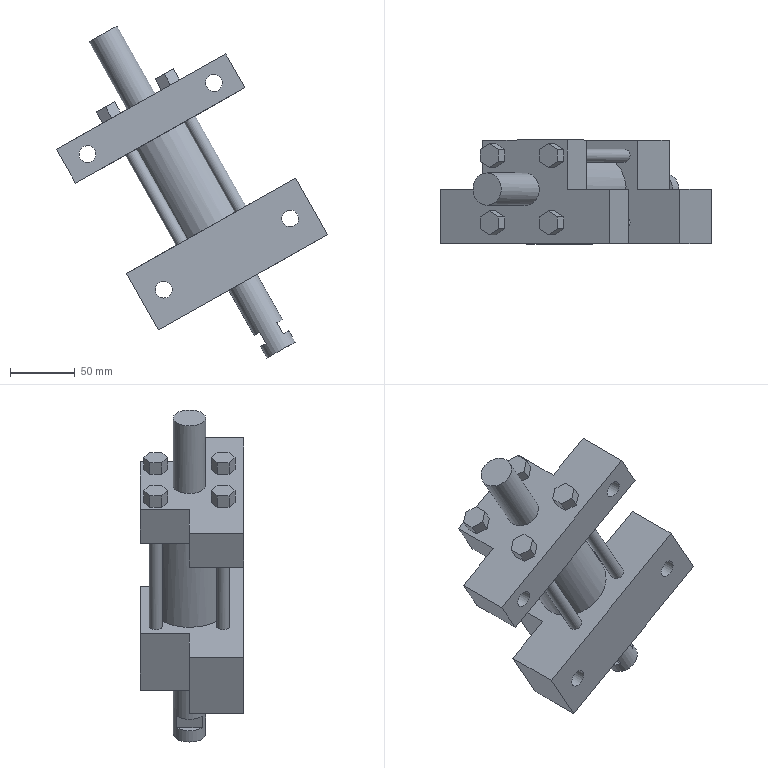Part | STEP file | solid 157 | 1 solid | 79 faces | box 209.196 x 80 x 256.267 mm | volume 975283 mm3 | plane 60 | cylinder 17 | cone 2 | commonest cylinder face diameters 10 x4 13 x4 20 x4 15 x2 25 x2 55 x1